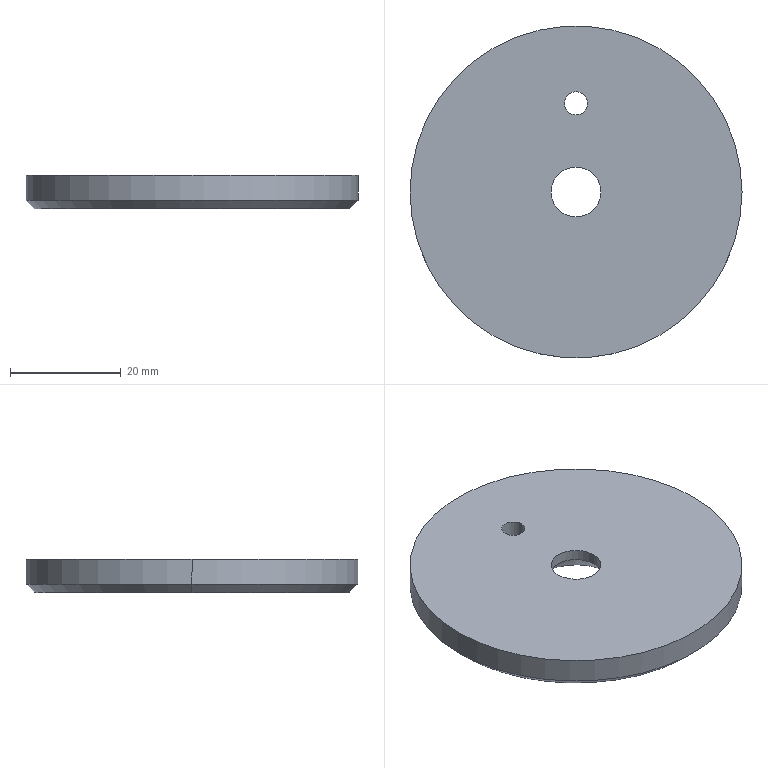Part | SolidWorks | features BaseBody 1 | 1 solid | 12 faces | box 60 x 60 x 6 mm | volume 15998 mm3 | cylinder 6 | cone 4 | plane 2 | commonest cylinder face diameters 4.2 x2 9 x2 60 x2
STEP:
#1=CARTESIAN_POINT('',(2.1,16.,6.));
#2=VERTEX_POINT('',#1);
#3=CARTESIAN_POINT('',(-2.1,16.,6.));
#4=VERTEX_POINT('',#3);
#5=CARTESIAN_POINT('',(0.,16.,6.));
#6=DIRECTION('',(0.,0.,-1.));
#7=DIRECTION('',(-1.,0.,0.));
#8=AXIS2_PLACEMENT_3D('',#5,#6,#7);
#9=CIRCLE('',#8,2.1);
#10=EDGE_CURVE('',#2,#4,#9,.T.);
#11=ORIENTED_EDGE('',*,*,#10,.F.);
#12=CARTESIAN_POINT('',(2.1,16.,0.));
#13=VERTEX_POINT('',#12);
#14=CARTESIAN_POINT('',(2.1,16.,6.));
#15=DIRECTION('',(0.,0.,-1.));
#16=VECTOR('',#15,1000.);
#17=LINE('',#14,#16);
#18=EDGE_CURVE('',#2,#13,#17,.T.);
#19=ORIENTED_EDGE('',*,*,#18,.T.);
#20=CARTESIAN_POINT('',(-2.1,16.,0.));
#21=VERTEX_POINT('',#20);
#22=CARTESIAN_POINT('',(0.,16.,0.));
#23=DIRECTION('',(0.,0.,1.));
#24=DIRECTION('',(-1.,0.,0.));
#25=AXIS2_PLACEMENT_3D('',#22,#23,#24);
#26=CIRCLE('',#25,2.1);
#27=EDGE_CURVE('',#21,#13,#26,.T.);
#28=ORIENTED_EDGE('',*,*,#27,.F.);
#29=CARTESIAN_POINT('',(-2.1,16.,6.));
#30=DIRECTION('',(0.,0.,-1.));
#31=VECTOR('',#30,1000.);
#32=LINE('',#29,#31);
#33=EDGE_CURVE('',#4,#21,#32,.T.);
#34=ORIENTED_EDGE('',*,*,#33,.F.);
#35=EDGE_LOOP('',(#11,#19,#28,#34));
#36=FACE_OUTER_BOUND('',#35,.T.);
#37=CARTESIAN_POINT('',(0.,16.,6.));
#38=DIRECTION('',(0.,0.,-1.));
#39=DIRECTION('',(-1.,0.,0.));
#40=AXIS2_PLACEMENT_3D('',#37,#38,#39);
#41=CYLINDRICAL_SURFACE('',#40,2.1);
#42=ADVANCED_FACE('',(#36),#41,.F.);
#43=CARTESIAN_POINT('',(30.,0.,6.));
#44=VERTEX_POINT('',#43);
#45=CARTESIAN_POINT('',(-30.,0.,6.));
#46=VERTEX_POINT('',#45);
#47=CARTESIAN_POINT('',(0.,0.,6.));
#48=DIRECTION('',(0.,0.,1.));
#49=DIRECTION('',(-1.,0.,0.));
#50=AXIS2_PLACEMENT_3D('',#47,#48,#49);
#51=CIRCLE('',#50,30.);
#52=EDGE_CURVE('',#44,#46,#51,.T.);
#53=ORIENTED_EDGE('',*,*,#52,.F.);
#54=CARTESIAN_POINT('',(30.,0.,1.5));
#55=VERTEX_POINT('',#54);
#56=CARTESIAN_POINT('',(30.,0.,6.));
#57=DIRECTION('',(0.,0.,-1.));
#58=VECTOR('',#57,1000.);
#59=LINE('',#56,#58);
#60=EDGE_CURVE('',#44,#55,#59,.T.);
#61=ORIENTED_EDGE('',*,*,#60,.T.);
#62=CARTESIAN_POINT('',(-30.,0.,1.5));
#63=VERTEX_POINT('',#62);
#64=CARTESIAN_POINT('',(0.,0.,1.5));
#65=DIRECTION('',(0.,0.,1.));
#66=DIRECTION('',(-1.,0.,0.));
#67=AXIS2_PLACEMENT_3D('',#64,#65,#66);
#68=CIRCLE('',#67,30.);
#69=EDGE_CURVE('',#55,#63,#68,.T.);
#70=ORIENTED_EDGE('',*,*,#69,.T.);
#71=CARTESIAN_POINT('',(-30.,0.,6.));
#72=DIRECTION('',(0.,0.,-1.));
#73=VECTOR('',#72,1000.);
#74=LINE('',#71,#73);
#75=EDGE_CURVE('',#46,#63,#74,.T.);
#76=ORIENTED_EDGE('',*,*,#75,.F.);
#77=EDGE_LOOP('',(#53,#61,#70,#76));
#78=FACE_OUTER_BOUND('',#77,.T.);
#79=CARTESIAN_POINT('',(0.,0.,6.));
#80=DIRECTION('',(0.,0.,-1.));
#81=DIRECTION('',(-1.,0.,0.));
#82=AXIS2_PLACEMENT_3D('',#79,#80,#81);
#83=CYLINDRICAL_SURFACE('',#82,30.);
#84=ADVANCED_FACE('',(#78),#83,.T.);
#85=CARTESIAN_POINT('',(4.5,0.,6.));
#86=VERTEX_POINT('',#85);
#87=CARTESIAN_POINT('',(-4.5,0.,6.));
#88=VERTEX_POINT('',#87);
#89=CARTESIAN_POINT('',(0.,0.,6.));
#90=DIRECTION('',(0.,0.,-1.));
#91=DIRECTION('',(-1.,0.,0.));
#92=AXIS2_PLACEMENT_3D('',#89,#90,#91);
#93=CIRCLE('',#92,4.5);
#94=EDGE_CURVE('',#86,#88,#93,.T.);
#95=ORIENTED_EDGE('',*,*,#94,.F.);
#96=CARTESIAN_POINT('',(4.5,0.,4.));
#97=VERTEX_POINT('',#96);
#98=CARTESIAN_POINT('',(4.5,0.,6.));
#99=DIRECTION('',(0.,0.,-1.));
#100=VECTOR('',#99,1000.);
#101=LINE('',#98,#100);
#102=EDGE_CURVE('',#86,#97,#101,.T.);
#103=ORIENTED_EDGE('',*,*,#102,.T.);
#104=CARTESIAN_POINT('',(-4.5,0.,4.));
#105=VERTEX_POINT('',#104);
#106=CARTESIAN_POINT('',(0.,0.,4.));
#107=DIRECTION('',(0.,0.,1.));
#108=DIRECTION('',(-1.,0.,0.));
#109=AXIS2_PLACEMENT_3D('',#106,#107,#108);
#110=CIRCLE('',#109,4.5);
#111=EDGE_CURVE('',#105,#97,#110,.T.);
#112=ORIENTED_EDGE('',*,*,#111,.F.);
#113=CARTESIAN_POINT('',(-4.5,0.,6.));
#114=DIRECTION('',(0.,0.,-1.));
#115=VECTOR('',#114,1000.);
#116=LINE('',#113,#115);
#117=EDGE_CURVE('',#88,#105,#116,.T.);
#118=ORIENTED_EDGE('',*,*,#117,.F.);
#119=EDGE_LOOP('',(#95,#103,#112,#118));
#120=FACE_OUTER_BOUND('',#119,.T.);
#121=CARTESIAN_POINT('',(0.,0.,6.));
#122=DIRECTION('',(0.,0.,-1.));
#123=DIRECTION('',(-1.,0.,0.));
#124=AXIS2_PLACEMENT_3D('',#121,#122,#123);
#125=CYLINDRICAL_SURFACE('',#124,4.5);
#126=ADVANCED_FACE('',(#120),#125,.F.);
#127=CARTESIAN_POINT('',(28.5,0.,0.));
#128=VERTEX_POINT('',#127);
#129=CARTESIAN_POINT('',(-28.5,0.,0.));
#130=VERTEX_POINT('',#129);
#131=CARTESIAN_POINT('',(0.,0.,0.));
#132=DIRECTION('',(0.,0.,1.));
#133=DIRECTION('',(1.,0.,0.));
#134=AXIS2_PLACEMENT_3D('',#131,#132,#133);
#135=CIRCLE('',#134,28.5);
#136=EDGE_CURVE('',#128,#130,#135,.T.);
#137=ORIENTED_EDGE('',*,*,#136,.T.);
#138=CARTESIAN_POINT('',(-30.,0.,1.5));
#139=DIRECTION('',(-0.7071,0.,0.7071));
#140=VECTOR('',#139,1000.);
#141=LINE('',#138,#140);
#142=EDGE_CURVE('',#130,#63,#141,.T.);
#143=ORIENTED_EDGE('',*,*,#142,.T.);
#144=ORIENTED_EDGE('',*,*,#69,.F.);
#145=CARTESIAN_POINT('',(30.,0.,1.5));
#146=DIRECTION('',(0.7071,0.,0.7071));
#147=VECTOR('',#146,1000.);
#148=LINE('',#145,#147);
#149=EDGE_CURVE('',#128,#55,#148,.T.);
#150=ORIENTED_EDGE('',*,*,#149,.F.);
#151=EDGE_LOOP('',(#137,#143,#144,#150));
#152=FACE_OUTER_BOUND('',#151,.T.);
#153=CARTESIAN_POINT('',(0.,0.,1.5));
#154=DIRECTION('',(0.,0.,1.));
#155=DIRECTION('',(1.,0.,0.));
#156=AXIS2_PLACEMENT_3D('',#153,#154,#155);
#157=CONICAL_SURFACE('',#156,30.,0.7854);
#158=ADVANCED_FACE('',(#152),#157,.T.);
#159=ORIENTED_EDGE('',*,*,#111,.T.);
#160=CARTESIAN_POINT('',(8.5,0.,0.));
#161=VERTEX_POINT('',#160);
#162=CARTESIAN_POINT('',(8.5,0.,0.));
#163=DIRECTION('',(0.7071,0.,-0.7071));
#164=VECTOR('',#163,1000.);
#165=LINE('',#162,#164);
#166=EDGE_CURVE('',#97,#161,#165,.T.);
#167=ORIENTED_EDGE('',*,*,#166,.T.);
#168=CARTESIAN_POINT('',(-8.5,0.,0.));
#169=VERTEX_POINT('',#168);
#170=CARTESIAN_POINT('',(0.,0.,0.));
#171=DIRECTION('',(0.,0.,-1.));
#172=DIRECTION('',(-1.,0.,0.));
#173=AXIS2_PLACEMENT_3D('',#170,#171,#172);
#174=CIRCLE('',#173,8.5);
#175=EDGE_CURVE('',#161,#169,#174,.T.);
#176=ORIENTED_EDGE('',*,*,#175,.T.);
#177=CARTESIAN_POINT('',(-8.5,0.,0.));
#178=DIRECTION('',(-0.7071,0.,-0.7071));
#179=VECTOR('',#178,1000.);
#180=LINE('',#177,#179);
#181=EDGE_CURVE('',#105,#169,#180,.T.);
#182=ORIENTED_EDGE('',*,*,#181,.F.);
#183=EDGE_LOOP('',(#159,#167,#176,#182));
#184=FACE_OUTER_BOUND('',#183,.T.);
#185=CARTESIAN_POINT('',(0.,0.,0.));
#186=DIRECTION('',(0.,0.,-1.));
#187=DIRECTION('',(-1.,0.,0.));
#188=AXIS2_PLACEMENT_3D('',#185,#186,#187);
#189=CONICAL_SURFACE('',#188,8.5,0.7854);
#190=ADVANCED_FACE('',(#184),#189,.F.);
#191=CARTESIAN_POINT('',(0.,16.,6.));
#192=DIRECTION('',(0.,0.,-1.));
#193=DIRECTION('',(-1.,0.,0.));
#194=AXIS2_PLACEMENT_3D('',#191,#192,#193);
#195=CIRCLE('',#194,2.1);
#196=EDGE_CURVE('',#4,#2,#195,.T.);
#197=ORIENTED_EDGE('',*,*,#196,.T.);
#198=ORIENTED_EDGE('',*,*,#10,.T.);
#199=EDGE_LOOP('',(#197,#198));
#200=FACE_BOUND('',#199,.T.);
#201=CARTESIAN_POINT('',(0.,0.,6.));
#202=DIRECTION('',(0.,0.,1.));
#203=DIRECTION('',(-1.,0.,0.));
#204=AXIS2_PLACEMENT_3D('',#201,#202,#203);
#205=CIRCLE('',#204,30.);
#206=EDGE_CURVE('',#46,#44,#205,.T.);
#207=ORIENTED_EDGE('',*,*,#206,.T.);
#208=ORIENTED_EDGE('',*,*,#52,.T.);
#209=EDGE_LOOP('',(#207,#208));
#210=FACE_OUTER_BOUND('',#209,.T.);
#211=CARTESIAN_POINT('',(0.,0.,6.));
#212=DIRECTION('',(0.,0.,-1.));
#213=DIRECTION('',(-1.,0.,0.));
#214=AXIS2_PLACEMENT_3D('',#211,#212,#213);
#215=CIRCLE('',#214,4.5);
#216=EDGE_CURVE('',#88,#86,#215,.T.);
#217=ORIENTED_EDGE('',*,*,#216,.T.);
#218=ORIENTED_EDGE('',*,*,#94,.T.);
#219=EDGE_LOOP('',(#217,#218));
#220=FACE_BOUND('',#219,.T.);
#221=CARTESIAN_POINT('',(0.,0.,6.));
#222=DIRECTION('',(0.,0.,1.));
#223=DIRECTION('',(1.,0.,0.));
#224=AXIS2_PLACEMENT_3D('',#221,#222,#223);
#225=PLANE('',#224);
#226=ADVANCED_FACE('',(#200,#210,#220),#225,.T.);
#227=ORIENTED_EDGE('',*,*,#18,.F.);
#228=ORIENTED_EDGE('',*,*,#196,.F.);
#229=ORIENTED_EDGE('',*,*,#33,.T.);
#230=CARTESIAN_POINT('',(0.,16.,0.));
#231=DIRECTION('',(0.,0.,1.));
#232=DIRECTION('',(-1.,0.,0.));
#233=AXIS2_PLACEMENT_3D('',#230,#231,#232);
#234=CIRCLE('',#233,2.1);
#235=EDGE_CURVE('',#13,#21,#234,.T.);
#236=ORIENTED_EDGE('',*,*,#235,.F.);
#237=EDGE_LOOP('',(#227,#228,#229,#236));
#238=FACE_OUTER_BOUND('',#237,.T.);
#239=CARTESIAN_POINT('',(0.,16.,6.));
#240=DIRECTION('',(0.,0.,-1.));
#241=DIRECTION('',(-1.,0.,0.));
#242=AXIS2_PLACEMENT_3D('',#239,#240,#241);
#243=CYLINDRICAL_SURFACE('',#242,2.1);
#244=ADVANCED_FACE('',(#238),#243,.F.);
#245=ORIENTED_EDGE('',*,*,#60,.F.);
#246=ORIENTED_EDGE('',*,*,#206,.F.);
#247=ORIENTED_EDGE('',*,*,#75,.T.);
#248=CARTESIAN_POINT('',(0.,0.,1.5));
#249=DIRECTION('',(0.,0.,1.));
#250=DIRECTION('',(-1.,0.,0.));
#251=AXIS2_PLACEMENT_3D('',#248,#249,#250);
#252=CIRCLE('',#251,30.);
#253=EDGE_CURVE('',#63,#55,#252,.T.);
#254=ORIENTED_EDGE('',*,*,#253,.T.);
#255=EDGE_LOOP('',(#245,#246,#247,#254));
#256=FACE_OUTER_BOUND('',#255,.T.);
#257=CARTESIAN_POINT('',(0.,0.,6.));
#258=DIRECTION('',(0.,0.,-1.));
#259=DIRECTION('',(-1.,0.,0.));
#260=AXIS2_PLACEMENT_3D('',#257,#258,#259);
#261=CYLINDRICAL_SURFACE('',#260,30.);
#262=ADVANCED_FACE('',(#256),#261,.T.);
#263=ORIENTED_EDGE('',*,*,#102,.F.);
#264=ORIENTED_EDGE('',*,*,#216,.F.);
#265=ORIENTED_EDGE('',*,*,#117,.T.);
#266=CARTESIAN_POINT('',(0.,0.,4.));
#267=DIRECTION('',(0.,0.,1.));
#268=DIRECTION('',(-1.,0.,0.));
#269=AXIS2_PLACEMENT_3D('',#266,#267,#268);
#270=CIRCLE('',#269,4.5);
#271=EDGE_CURVE('',#97,#105,#270,.T.);
#272=ORIENTED_EDGE('',*,*,#271,.F.);
#273=EDGE_LOOP('',(#263,#264,#265,#272));
#274=FACE_OUTER_BOUND('',#273,.T.);
#275=CARTESIAN_POINT('',(0.,0.,6.));
#276=DIRECTION('',(0.,0.,-1.));
#277=DIRECTION('',(-1.,0.,0.));
#278=AXIS2_PLACEMENT_3D('',#275,#276,#277);
#279=CYLINDRICAL_SURFACE('',#278,4.5);
#280=ADVANCED_FACE('',(#274),#279,.F.);
#281=ORIENTED_EDGE('',*,*,#27,.T.);
#282=ORIENTED_EDGE('',*,*,#235,.T.);
#283=EDGE_LOOP('',(#281,#282));
#284=FACE_BOUND('',#283,.T.);
#285=CARTESIAN_POINT('',(0.,0.,0.));
#286=DIRECTION('',(0.,0.,-1.));
#287=DIRECTION('',(-1.,0.,0.));
#288=AXIS2_PLACEMENT_3D('',#285,#286,#287);
#289=CIRCLE('',#288,8.5);
#290=EDGE_CURVE('',#169,#161,#289,.T.);
#291=ORIENTED_EDGE('',*,*,#290,.F.);
#292=ORIENTED_EDGE('',*,*,#175,.F.);
#293=EDGE_LOOP('',(#291,#292));
#294=FACE_BOUND('',#293,.T.);
#295=ORIENTED_EDGE('',*,*,#136,.F.);
#296=CARTESIAN_POINT('',(0.,0.,0.));
#297=DIRECTION('',(0.,0.,1.));
#298=DIRECTION('',(1.,0.,0.));
#299=AXIS2_PLACEMENT_3D('',#296,#297,#298);
#300=CIRCLE('',#299,28.5);
#301=EDGE_CURVE('',#130,#128,#300,.T.);
#302=ORIENTED_EDGE('',*,*,#301,.F.);
#303=EDGE_LOOP('',(#295,#302));
#304=FACE_OUTER_BOUND('',#303,.T.);
#305=CARTESIAN_POINT('',(0.,0.,0.));
#306=DIRECTION('',(0.,0.,1.));
#307=DIRECTION('',(1.,0.,0.));
#308=AXIS2_PLACEMENT_3D('',#305,#306,#307);
#309=PLANE('',#308);
#310=ADVANCED_FACE('',(#284,#294,#304),#309,.F.);
#311=ORIENTED_EDGE('',*,*,#142,.F.);
#312=ORIENTED_EDGE('',*,*,#301,.T.);
#313=ORIENTED_EDGE('',*,*,#149,.T.);
#314=ORIENTED_EDGE('',*,*,#253,.F.);
#315=EDGE_LOOP('',(#311,#312,#313,#314));
#316=FACE_OUTER_BOUND('',#315,.T.);
#317=CARTESIAN_POINT('',(0.,0.,1.5));
#318=DIRECTION('',(0.,0.,1.));
#319=DIRECTION('',(1.,0.,0.));
#320=AXIS2_PLACEMENT_3D('',#317,#318,#319);
#321=CONICAL_SURFACE('',#320,30.,0.7854);
#322=ADVANCED_FACE('',(#316),#321,.T.);
#323=ORIENTED_EDGE('',*,*,#166,.F.);
#324=ORIENTED_EDGE('',*,*,#271,.T.);
#325=ORIENTED_EDGE('',*,*,#181,.T.);
#326=ORIENTED_EDGE('',*,*,#290,.T.);
#327=EDGE_LOOP('',(#323,#324,#325,#326));
#328=FACE_OUTER_BOUND('',#327,.T.);
#329=CARTESIAN_POINT('',(0.,0.,0.));
#330=DIRECTION('',(0.,0.,-1.));
#331=DIRECTION('',(-1.,0.,0.));
#332=AXIS2_PLACEMENT_3D('',#329,#330,#331);
#333=CONICAL_SURFACE('',#332,8.5,0.7854);
#334=ADVANCED_FACE('',(#328),#333,.F.);
#335=CLOSED_SHELL('',(#42,#84,#126,#158,#190,#226,#244,#262,#280,#310,#322,#334));
#336=MANIFOLD_SOLID_BREP('',#335);
#337=CARTESIAN_POINT('',(0.,0.,0.));
#338=DIRECTION('',(0.,0.,1.));
#339=DIRECTION('',(1.,0.,0.));
#340=AXIS2_PLACEMENT_3D('',#337,#338,#339);
#341=(LENGTH_UNIT()NAMED_UNIT(*)SI_UNIT(.MILLI.,.METRE.));
#342=UNCERTAINTY_MEASURE_WITH_UNIT(LENGTH_MEASURE(0.00001),#341,'','');
#343=(NAMED_UNIT(*)PLANE_ANGLE_UNIT()SI_UNIT($,.RADIAN.));
#344=(NAMED_UNIT(*)SI_UNIT($,.STERADIAN.)SOLID_ANGLE_UNIT());
#345=(GEOMETRIC_REPRESENTATION_CONTEXT(3)GLOBAL_UNCERTAINTY_ASSIGNED_CONTEXT((#342))GLOBAL_UNIT_ASSIGNED_CONTEXT((#341,#343,#344))REPRESENTATION_CONTEXT('',''));
#346=ADVANCED_BREP_SHAPE_REPRESENTATION('',(#336,#340),#345);